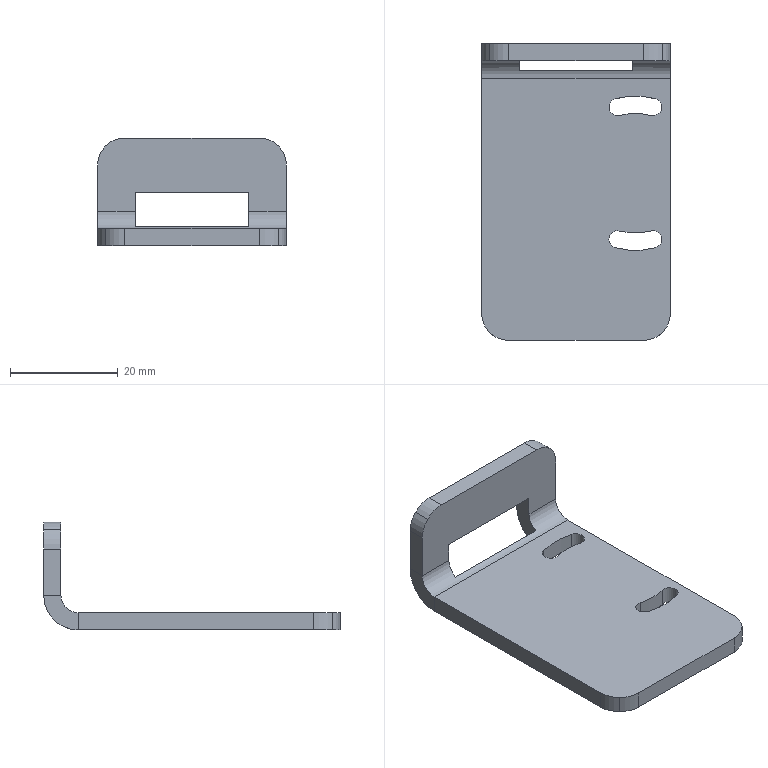Part | STEP file | DCV-000-016 | 1 solid | 36 faces | box 35 x 55 x 20 mm | volume 6902 mm3 | cylinder 19 | plane 17 | commonest cylinder face diameters 10 x8 3.2 x5 22.2 x2 28.6 x2 6.4 x1 12.8 x1